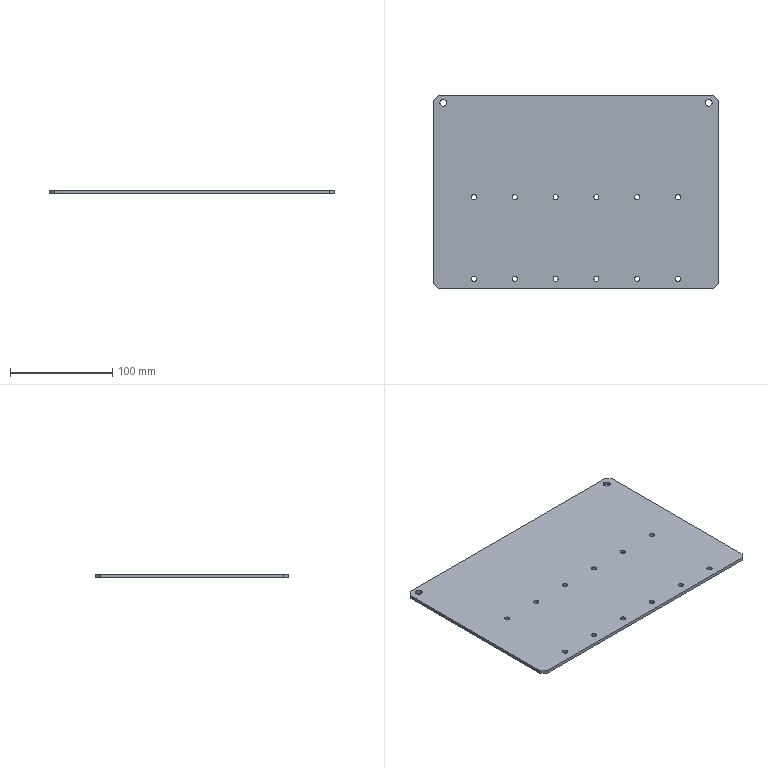Part | STEP file | J014-EBZ05-12-06-Part-1 | 1 solid | 38 faces | box 280 x 190 x 3.2 mm | volume 169094 mm3 | cylinder 28 | plane 10 | commonest cylinder face diameters 5 x24 6.8 x4
STEP:
#1=CARTESIAN_POINT('',(240.,12.5,3.2));
#2=VERTEX_POINT('',#1);
#3=CARTESIAN_POINT('',(240.,7.5,3.2));
#4=VERTEX_POINT('',#3);
#5=CARTESIAN_POINT('',(240.,10.,3.2));
#6=DIRECTION('',(0.,0.,-1.));
#7=DIRECTION('',(0.,-1.,0.));
#8=AXIS2_PLACEMENT_3D('',#5,#6,#7);
#9=CIRCLE('',#8,2.5);
#10=EDGE_CURVE('',#2,#4,#9,.T.);
#11=ORIENTED_EDGE('',*,*,#10,.F.);
#12=CARTESIAN_POINT('',(240.,12.5,0.));
#13=VERTEX_POINT('',#12);
#14=CARTESIAN_POINT('',(240.,12.5,3.2));
#15=DIRECTION('',(0.,0.,-1.));
#16=VECTOR('',#15,1000.);
#17=LINE('',#14,#16);
#18=EDGE_CURVE('',#2,#13,#17,.T.);
#19=ORIENTED_EDGE('',*,*,#18,.T.);
#20=CARTESIAN_POINT('',(240.,7.5,0.));
#21=VERTEX_POINT('',#20);
#22=CARTESIAN_POINT('',(240.,10.,0.));
#23=DIRECTION('',(0.,0.,1.));
#24=DIRECTION('',(0.,1.,0.));
#25=AXIS2_PLACEMENT_3D('',#22,#23,#24);
#26=CIRCLE('',#25,2.5);
#27=EDGE_CURVE('',#21,#13,#26,.T.);
#28=ORIENTED_EDGE('',*,*,#27,.F.);
#29=CARTESIAN_POINT('',(240.,7.5,3.2));
#30=DIRECTION('',(0.,0.,-1.));
#31=VECTOR('',#30,1000.);
#32=LINE('',#29,#31);
#33=EDGE_CURVE('',#4,#21,#32,.T.);
#34=ORIENTED_EDGE('',*,*,#33,.F.);
#35=EDGE_LOOP('',(#11,#19,#28,#34));
#36=FACE_OUTER_BOUND('',#35,.T.);
#37=CARTESIAN_POINT('',(240.,10.,3.2));
#38=DIRECTION('',(0.,0.,-1.));
#39=DIRECTION('',(0.,-1.,0.));
#40=AXIS2_PLACEMENT_3D('',#37,#38,#39);
#41=CYLINDRICAL_SURFACE('',#40,2.5);
#42=ADVANCED_FACE('',(#36),#41,.F.);
#43=CARTESIAN_POINT('',(240.,92.5,3.2));
#44=VERTEX_POINT('',#43);
#45=CARTESIAN_POINT('',(240.,87.5,3.2));
#46=VERTEX_POINT('',#45);
#47=CARTESIAN_POINT('',(240.,90.,3.2));
#48=DIRECTION('',(0.,0.,-1.));
#49=DIRECTION('',(0.,-1.,0.));
#50=AXIS2_PLACEMENT_3D('',#47,#48,#49);
#51=CIRCLE('',#50,2.5);
#52=EDGE_CURVE('',#44,#46,#51,.T.);
#53=ORIENTED_EDGE('',*,*,#52,.F.);
#54=CARTESIAN_POINT('',(240.,92.5,0.));
#55=VERTEX_POINT('',#54);
#56=CARTESIAN_POINT('',(240.,92.5,3.2));
#57=DIRECTION('',(0.,0.,-1.));
#58=VECTOR('',#57,1000.);
#59=LINE('',#56,#58);
#60=EDGE_CURVE('',#44,#55,#59,.T.);
#61=ORIENTED_EDGE('',*,*,#60,.T.);
#62=CARTESIAN_POINT('',(240.,87.5,0.));
#63=VERTEX_POINT('',#62);
#64=CARTESIAN_POINT('',(240.,90.,0.));
#65=DIRECTION('',(0.,0.,1.));
#66=DIRECTION('',(0.,1.,0.));
#67=AXIS2_PLACEMENT_3D('',#64,#65,#66);
#68=CIRCLE('',#67,2.5);
#69=EDGE_CURVE('',#63,#55,#68,.T.);
#70=ORIENTED_EDGE('',*,*,#69,.F.);
#71=CARTESIAN_POINT('',(240.,87.5,3.2));
#72=DIRECTION('',(0.,0.,-1.));
#73=VECTOR('',#72,1000.);
#74=LINE('',#71,#73);
#75=EDGE_CURVE('',#46,#63,#74,.T.);
#76=ORIENTED_EDGE('',*,*,#75,.F.);
#77=EDGE_LOOP('',(#53,#61,#70,#76));
#78=FACE_OUTER_BOUND('',#77,.T.);
#79=CARTESIAN_POINT('',(240.,90.,3.2));
#80=DIRECTION('',(0.,0.,-1.));
#81=DIRECTION('',(0.,-1.,0.));
#82=AXIS2_PLACEMENT_3D('',#79,#80,#81);
#83=CYLINDRICAL_SURFACE('',#82,2.5);
#84=ADVANCED_FACE('',(#78),#83,.F.);
#85=CARTESIAN_POINT('',(200.,12.5,3.2));
#86=VERTEX_POINT('',#85);
#87=CARTESIAN_POINT('',(200.,7.5,3.2));
#88=VERTEX_POINT('',#87);
#89=CARTESIAN_POINT('',(200.,10.,3.2));
#90=DIRECTION('',(0.,0.,-1.));
#91=DIRECTION('',(0.,-1.,0.));
#92=AXIS2_PLACEMENT_3D('',#89,#90,#91);
#93=CIRCLE('',#92,2.5);
#94=EDGE_CURVE('',#86,#88,#93,.T.);
#95=ORIENTED_EDGE('',*,*,#94,.F.);
#96=CARTESIAN_POINT('',(200.,12.5,0.));
#97=VERTEX_POINT('',#96);
#98=CARTESIAN_POINT('',(200.,12.5,3.2));
#99=DIRECTION('',(0.,0.,-1.));
#100=VECTOR('',#99,1000.);
#101=LINE('',#98,#100);
#102=EDGE_CURVE('',#86,#97,#101,.T.);
#103=ORIENTED_EDGE('',*,*,#102,.T.);
#104=CARTESIAN_POINT('',(200.,7.5,0.));
#105=VERTEX_POINT('',#104);
#106=CARTESIAN_POINT('',(200.,10.,0.));
#107=DIRECTION('',(0.,0.,1.));
#108=DIRECTION('',(0.,1.,0.));
#109=AXIS2_PLACEMENT_3D('',#106,#107,#108);
#110=CIRCLE('',#109,2.5);
#111=EDGE_CURVE('',#105,#97,#110,.T.);
#112=ORIENTED_EDGE('',*,*,#111,.F.);
#113=CARTESIAN_POINT('',(200.,7.5,3.2));
#114=DIRECTION('',(0.,0.,-1.));
#115=VECTOR('',#114,1000.);
#116=LINE('',#113,#115);
#117=EDGE_CURVE('',#88,#105,#116,.T.);
#118=ORIENTED_EDGE('',*,*,#117,.F.);
#119=EDGE_LOOP('',(#95,#103,#112,#118));
#120=FACE_OUTER_BOUND('',#119,.T.);
#121=CARTESIAN_POINT('',(200.,10.,3.2));
#122=DIRECTION('',(0.,0.,-1.));
#123=DIRECTION('',(0.,-1.,0.));
#124=AXIS2_PLACEMENT_3D('',#121,#122,#123);
#125=CYLINDRICAL_SURFACE('',#124,2.5);
#126=ADVANCED_FACE('',(#120),#125,.F.);
#127=CARTESIAN_POINT('',(200.,92.5,3.2));
#128=VERTEX_POINT('',#127);
#129=CARTESIAN_POINT('',(200.,87.5,3.2));
#130=VERTEX_POINT('',#129);
#131=CARTESIAN_POINT('',(200.,90.,3.2));
#132=DIRECTION('',(0.,0.,-1.));
#133=DIRECTION('',(0.,-1.,0.));
#134=AXIS2_PLACEMENT_3D('',#131,#132,#133);
#135=CIRCLE('',#134,2.5);
#136=EDGE_CURVE('',#128,#130,#135,.T.);
#137=ORIENTED_EDGE('',*,*,#136,.F.);
#138=CARTESIAN_POINT('',(200.,92.5,0.));
#139=VERTEX_POINT('',#138);
#140=CARTESIAN_POINT('',(200.,92.5,3.2));
#141=DIRECTION('',(0.,0.,-1.));
#142=VECTOR('',#141,1000.);
#143=LINE('',#140,#142);
#144=EDGE_CURVE('',#128,#139,#143,.T.);
#145=ORIENTED_EDGE('',*,*,#144,.T.);
#146=CARTESIAN_POINT('',(200.,87.5,0.));
#147=VERTEX_POINT('',#146);
#148=CARTESIAN_POINT('',(200.,90.,0.));
#149=DIRECTION('',(0.,0.,1.));
#150=DIRECTION('',(0.,1.,0.));
#151=AXIS2_PLACEMENT_3D('',#148,#149,#150);
#152=CIRCLE('',#151,2.5);
#153=EDGE_CURVE('',#147,#139,#152,.T.);
#154=ORIENTED_EDGE('',*,*,#153,.F.);
#155=CARTESIAN_POINT('',(200.,87.5,3.2));
#156=DIRECTION('',(0.,0.,-1.));
#157=VECTOR('',#156,1000.);
#158=LINE('',#155,#157);
#159=EDGE_CURVE('',#130,#147,#158,.T.);
#160=ORIENTED_EDGE('',*,*,#159,.F.);
#161=EDGE_LOOP('',(#137,#145,#154,#160));
#162=FACE_OUTER_BOUND('',#161,.T.);
#163=CARTESIAN_POINT('',(200.,90.,3.2));
#164=DIRECTION('',(0.,0.,-1.));
#165=DIRECTION('',(0.,-1.,0.));
#166=AXIS2_PLACEMENT_3D('',#163,#164,#165);
#167=CYLINDRICAL_SURFACE('',#166,2.5);
#168=ADVANCED_FACE('',(#162),#167,.F.);
#169=CARTESIAN_POINT('',(160.,12.5,3.2));
#170=VERTEX_POINT('',#169);
#171=CARTESIAN_POINT('',(160.,7.5,3.2));
#172=VERTEX_POINT('',#171);
#173=CARTESIAN_POINT('',(160.,10.,3.2));
#174=DIRECTION('',(0.,0.,-1.));
#175=DIRECTION('',(0.,-1.,0.));
#176=AXIS2_PLACEMENT_3D('',#173,#174,#175);
#177=CIRCLE('',#176,2.5);
#178=EDGE_CURVE('',#170,#172,#177,.T.);
#179=ORIENTED_EDGE('',*,*,#178,.F.);
#180=CARTESIAN_POINT('',(160.,12.5,0.));
#181=VERTEX_POINT('',#180);
#182=CARTESIAN_POINT('',(160.,12.5,3.2));
#183=DIRECTION('',(0.,0.,-1.));
#184=VECTOR('',#183,1000.);
#185=LINE('',#182,#184);
#186=EDGE_CURVE('',#170,#181,#185,.T.);
#187=ORIENTED_EDGE('',*,*,#186,.T.);
#188=CARTESIAN_POINT('',(160.,7.5,0.));
#189=VERTEX_POINT('',#188);
#190=CARTESIAN_POINT('',(160.,10.,0.));
#191=DIRECTION('',(0.,0.,1.));
#192=DIRECTION('',(0.,1.,0.));
#193=AXIS2_PLACEMENT_3D('',#190,#191,#192);
#194=CIRCLE('',#193,2.5);
#195=EDGE_CURVE('',#189,#181,#194,.T.);
#196=ORIENTED_EDGE('',*,*,#195,.F.);
#197=CARTESIAN_POINT('',(160.,7.5,3.2));
#198=DIRECTION('',(0.,0.,-1.));
#199=VECTOR('',#198,1000.);
#200=LINE('',#197,#199);
#201=EDGE_CURVE('',#172,#189,#200,.T.);
#202=ORIENTED_EDGE('',*,*,#201,.F.);
#203=EDGE_LOOP('',(#179,#187,#196,#202));
#204=FACE_OUTER_BOUND('',#203,.T.);
#205=CARTESIAN_POINT('',(160.,10.,3.2));
#206=DIRECTION('',(0.,0.,-1.));
#207=DIRECTION('',(0.,-1.,0.));
#208=AXIS2_PLACEMENT_3D('',#205,#206,#207);
#209=CYLINDRICAL_SURFACE('',#208,2.5);
#210=ADVANCED_FACE('',(#204),#209,.F.);
#211=CARTESIAN_POINT('',(160.,92.5,3.2));
#212=VERTEX_POINT('',#211);
#213=CARTESIAN_POINT('',(160.,87.5,3.2));
#214=VERTEX_POINT('',#213);
#215=CARTESIAN_POINT('',(160.,90.,3.2));
#216=DIRECTION('',(0.,0.,-1.));
#217=DIRECTION('',(0.,-1.,0.));
#218=AXIS2_PLACEMENT_3D('',#215,#216,#217);
#219=CIRCLE('',#218,2.5);
#220=EDGE_CURVE('',#212,#214,#219,.T.);
#221=ORIENTED_EDGE('',*,*,#220,.F.);
#222=CARTESIAN_POINT('',(160.,92.5,0.));
#223=VERTEX_POINT('',#222);
#224=CARTESIAN_POINT('',(160.,92.5,3.2));
#225=DIRECTION('',(0.,0.,-1.));
#226=VECTOR('',#225,1000.);
#227=LINE('',#224,#226);
#228=EDGE_CURVE('',#212,#223,#227,.T.);
#229=ORIENTED_EDGE('',*,*,#228,.T.);
#230=CARTESIAN_POINT('',(160.,87.5,0.));
#231=VERTEX_POINT('',#230);
#232=CARTESIAN_POINT('',(160.,90.,0.));
#233=DIRECTION('',(0.,0.,1.));
#234=DIRECTION('',(0.,1.,0.));
#235=AXIS2_PLACEMENT_3D('',#232,#233,#234);
#236=CIRCLE('',#235,2.5);
#237=EDGE_CURVE('',#231,#223,#236,.T.);
#238=ORIENTED_EDGE('',*,*,#237,.F.);
#239=CARTESIAN_POINT('',(160.,87.5,3.2));
#240=DIRECTION('',(0.,0.,-1.));
#241=VECTOR('',#240,1000.);
#242=LINE('',#239,#241);
#243=EDGE_CURVE('',#214,#231,#242,.T.);
#244=ORIENTED_EDGE('',*,*,#243,.F.);
#245=EDGE_LOOP('',(#221,#229,#238,#244));
#246=FACE_OUTER_BOUND('',#245,.T.);
#247=CARTESIAN_POINT('',(160.,90.,3.2));
#248=DIRECTION('',(0.,0.,-1.));
#249=DIRECTION('',(0.,-1.,0.));
#250=AXIS2_PLACEMENT_3D('',#247,#248,#249);
#251=CYLINDRICAL_SURFACE('',#250,2.5);
#252=ADVANCED_FACE('',(#246),#251,.F.);
#253=CARTESIAN_POINT('',(120.,12.5,3.2));
#254=VERTEX_POINT('',#253);
#255=CARTESIAN_POINT('',(120.,7.5,3.2));
#256=VERTEX_POINT('',#255);
#257=CARTESIAN_POINT('',(120.,10.,3.2));
#258=DIRECTION('',(0.,0.,-1.));
#259=DIRECTION('',(0.,-1.,0.));
#260=AXIS2_PLACEMENT_3D('',#257,#258,#259);
#261=CIRCLE('',#260,2.5);
#262=EDGE_CURVE('',#254,#256,#261,.T.);
#263=ORIENTED_EDGE('',*,*,#262,.F.);
#264=CARTESIAN_POINT('',(120.,12.5,0.));
#265=VERTEX_POINT('',#264);
#266=CARTESIAN_POINT('',(120.,12.5,3.2));
#267=DIRECTION('',(0.,0.,-1.));
#268=VECTOR('',#267,1000.);
#269=LINE('',#266,#268);
#270=EDGE_CURVE('',#254,#265,#269,.T.);
#271=ORIENTED_EDGE('',*,*,#270,.T.);
#272=CARTESIAN_POINT('',(120.,7.5,0.));
#273=VERTEX_POINT('',#272);
#274=CARTESIAN_POINT('',(120.,10.,0.));
#275=DIRECTION('',(0.,0.,1.));
#276=DIRECTION('',(0.,1.,0.));
#277=AXIS2_PLACEMENT_3D('',#274,#275,#276);
#278=CIRCLE('',#277,2.5);
#279=EDGE_CURVE('',#273,#265,#278,.T.);
#280=ORIENTED_EDGE('',*,*,#279,.F.);
#281=CARTESIAN_POINT('',(120.,7.5,3.2));
#282=DIRECTION('',(0.,0.,-1.));
#283=VECTOR('',#282,1000.);
#284=LINE('',#281,#283);
#285=EDGE_CURVE('',#256,#273,#284,.T.);
#286=ORIENTED_EDGE('',*,*,#285,.F.);
#287=EDGE_LOOP('',(#263,#271,#280,#286));
#288=FACE_OUTER_BOUND('',#287,.T.);
#289=CARTESIAN_POINT('',(120.,10.,3.2));
#290=DIRECTION('',(0.,0.,-1.));
#291=DIRECTION('',(0.,-1.,0.));
#292=AXIS2_PLACEMENT_3D('',#289,#290,#291);
#293=CYLINDRICAL_SURFACE('',#292,2.5);
#294=ADVANCED_FACE('',(#288),#293,.F.);
#295=CARTESIAN_POINT('',(120.,92.5,3.2));
#296=VERTEX_POINT('',#295);
#297=CARTESIAN_POINT('',(120.,87.5,3.2));
#298=VERTEX_POINT('',#297);
#299=CARTESIAN_POINT('',(120.,90.,3.2));
#300=DIRECTION('',(0.,0.,-1.));
#301=DIRECTION('',(0.,-1.,0.));
#302=AXIS2_PLACEMENT_3D('',#299,#300,#301);
#303=CIRCLE('',#302,2.5);
#304=EDGE_CURVE('',#296,#298,#303,.T.);
#305=ORIENTED_EDGE('',*,*,#304,.F.);
#306=CARTESIAN_POINT('',(120.,92.5,0.));
#307=VERTEX_POINT('',#306);
#308=CARTESIAN_POINT('',(120.,92.5,3.2));
#309=DIRECTION('',(0.,0.,-1.));
#310=VECTOR('',#309,1000.);
#311=LINE('',#308,#310);
#312=EDGE_CURVE('',#296,#307,#311,.T.);
#313=ORIENTED_EDGE('',*,*,#312,.T.);
#314=CARTESIAN_POINT('',(120.,87.5,0.));
#315=VERTEX_POINT('',#314);
#316=CARTESIAN_POINT('',(120.,90.,0.));
#317=DIRECTION('',(0.,0.,1.));
#318=DIRECTION('',(0.,1.,0.));
#319=AXIS2_PLACEMENT_3D('',#316,#317,#318);
#320=CIRCLE('',#319,2.5);
#321=EDGE_CURVE('',#315,#307,#320,.T.);
#322=ORIENTED_EDGE('',*,*,#321,.F.);
#323=CARTESIAN_POINT('',(120.,87.5,3.2));
#324=DIRECTION('',(0.,0.,-1.));
#325=VECTOR('',#324,1000.);
#326=LINE('',#323,#325);
#327=EDGE_CURVE('',#298,#315,#326,.T.);
#328=ORIENTED_EDGE('',*,*,#327,.F.);
#329=EDGE_LOOP('',(#305,#313,#322,#328));
#330=FACE_OUTER_BOUND('',#329,.T.);
#331=CARTESIAN_POINT('',(120.,90.,3.2));
#332=DIRECTION('',(0.,0.,-1.));
#333=DIRECTION('',(0.,-1.,0.));
#334=AXIS2_PLACEMENT_3D('',#331,#332,#333);
#335=CYLINDRICAL_SURFACE('',#334,2.5);
#336=ADVANCED_FACE('',(#330),#335,.F.);
#337=CARTESIAN_POINT('',(80.,12.5,3.2));
#338=VERTEX_POINT('',#337);
#339=CARTESIAN_POINT('',(80.,7.5,3.2));
#340=VERTEX_POINT('',#339);
#341=CARTESIAN_POINT('',(80.,10.,3.2));
#342=DIRECTION('',(0.,0.,-1.));
#343=DIRECTION('',(0.,-1.,0.));
#344=AXIS2_PLACEMENT_3D('',#341,#342,#343);
#345=CIRCLE('',#344,2.5);
#346=EDGE_CURVE('',#338,#340,#345,.T.);
#347=ORIENTED_EDGE('',*,*,#346,.F.);
#348=CARTESIAN_POINT('',(80.,12.5,0.));
#349=VERTEX_POINT('',#348);
#350=CARTESIAN_POINT('',(80.,12.5,3.2));
#351=DIRECTION('',(0.,0.,-1.));
#352=VECTOR('',#351,1000.);
#353=LINE('',#350,#352);
#354=EDGE_CURVE('',#338,#349,#353,.T.);
#355=ORIENTED_EDGE('',*,*,#354,.T.);
#356=CARTESIAN_POINT('',(80.,7.5,0.));
#357=VERTEX_POINT('',#356);
#358=CARTESIAN_POINT('',(80.,10.,0.));
#359=DIRECTION('',(0.,0.,1.));
#360=DIRECTION('',(0.,1.,0.));
#361=AXIS2_PLACEMENT_3D('',#358,#359,#360);
#362=CIRCLE('',#361,2.5);
#363=EDGE_CURVE('',#357,#349,#362,.T.);
#364=ORIENTED_EDGE('',*,*,#363,.F.);
#365=CARTESIAN_POINT('',(80.,7.5,3.2));
#366=DIRECTION('',(0.,0.,-1.));
#367=VECTOR('',#366,1000.);
#368=LINE('',#365,#367);
#369=EDGE_CURVE('',#340,#357,#368,.T.);
#370=ORIENTED_EDGE('',*,*,#369,.F.);
#371=EDGE_LOOP('',(#347,#355,#364,#370));
#372=FACE_OUTER_BOUND('',#371,.T.);
#373=CARTESIAN_POINT('',(80.,10.,3.2));
#374=DIRECTION('',(0.,0.,-1.));
#375=DIRECTION('',(0.,-1.,0.));
#376=AXIS2_PLACEMENT_3D('',#373,#374,#375);
#377=CYLINDRICAL_SURFACE('',#376,2.5);
#378=ADVANCED_FACE('',(#372),#377,.F.);
#379=CARTESIAN_POINT('',(80.,92.5,3.2));
#380=VERTEX_POINT('',#379);
#381=CARTESIAN_POINT('',(80.,87.5,3.2));
#382=VERTEX_POINT('',#381);
#383=CARTESIAN_POINT('',(80.,90.,3.2));
#384=DIRECTION('',(0.,0.,-1.));
#385=DIRECTION('',(0.,-1.,0.));
#386=AXIS2_PLACEMENT_3D('',#383,#384,#385);
#387=CIRCLE('',#386,2.5);
#388=EDGE_CURVE('',#380,#382,#387,.T.);
#389=ORIENTED_EDGE('',*,*,#388,.F.);
#390=CARTESIAN_POINT('',(80.,92.5,0.));
#391=VERTEX_POINT('',#390);
#392=CARTESIAN_POINT('',(80.,92.5,3.2));
#393=DIRECTION('',(0.,0.,-1.));
#394=VECTOR('',#393,1000.);
#395=LINE('',#392,#394);
#396=EDGE_CURVE('',#380,#391,#395,.T.);
#397=ORIENTED_EDGE('',*,*,#396,.T.);
#398=CARTESIAN_POINT('',(80.,87.5,0.));
#399=VERTEX_POINT('',#398);
#400=CARTESIAN_POINT('',(80.,90.,0.));
#401=DIRECTION('',(0.,0.,1.));
#402=DIRECTION('',(0.,1.,0.));
#403=AXIS2_PLACEMENT_3D('',#400,#401,#402);
#404=CIRCLE('',#403,2.5);
#405=EDGE_CURVE('',#399,#391,#404,.T.);
#406=ORIENTED_EDGE('',*,*,#405,.F.);
#407=CARTESIAN_POINT('',(80.,87.5,3.2));
#408=DIRECTION('',(0.,0.,-1.));
#409=VECTOR('',#408,1000.);
#410=LINE('',#407,#409);
#411=EDGE_CURVE('',#382,#399,#410,.T.);
#412=ORIENTED_EDGE('',*,*,#411,.F.);
#413=EDGE_LOOP('',(#389,#397,#406,#412));
#414=FACE_OUTER_BOUND('',#413,.T.);
#415=CARTESIAN_POINT('',(80.,90.,3.2));
#416=DIRECTION('',(0.,0.,-1.));
#417=DIRECTION('',(0.,-1.,0.));
#418=AXIS2_PLACEMENT_3D('',#415,#416,#417);
#419=CYLINDRICAL_SURFACE('',#418,2.5);
#420=ADVANCED_FACE('',(#414),#419,.F.);
#421=CARTESIAN_POINT('',(40.,12.5,3.2));
#422=VERTEX_POINT('',#421);
#423=CARTESIAN_POINT('',(40.,7.5,3.2));
#424=VERTEX_POINT('',#423);
#425=CARTESIAN_POINT('',(40.,10.,3.2));
#426=DIRECTION('',(0.,0.,-1.));
#427=DIRECTION('',(0.,-1.,0.));
#428=AXIS2_PLACEMENT_3D('',#425,#426,#427);
#429=CIRCLE('',#428,2.5);
#430=EDGE_CURVE('',#422,#424,#429,.T.);
#431=ORIENTED_EDGE('',*,*,#430,.F.);
#432=CARTESIAN_POINT('',(40.,12.5,0.));
#433=VERTEX_POINT('',#432);
#434=CARTESIAN_POINT('',(40.,12.5,3.2));
#435=DIRECTION('',(0.,0.,-1.));
#436=VECTOR('',#435,1000.);
#437=LINE('',#434,#436);
#438=EDGE_CURVE('',#422,#433,#437,.T.);
#439=ORIENTED_EDGE('',*,*,#438,.T.);
#440=CARTESIAN_POINT('',(40.,7.5,0.));
#441=VERTEX_POINT('',#440);
#442=CARTESIAN_POINT('',(40.,10.,0.));
#443=DIRECTION('',(0.,0.,1.));
#444=DIRECTION('',(0.,1.,0.));
#445=AXIS2_PLACEMENT_3D('',#442,#443,#444);
#446=CIRCLE('',#445,2.5);
#447=EDGE_CURVE('',#441,#433,#446,.T.);
#448=ORIENTED_EDGE('',*,*,#447,.F.);
#449=CARTESIAN_POINT('',(40.,7.5,3.2));
#450=DIRECTION('',(0.,0.,-1.));
#451=VECTOR('',#450,1000.);
#452=LINE('',#449,#451);
#453=EDGE_CURVE('',#424,#441,#452,.T.);
#454=ORIENTED_EDGE('',*,*,#453,.F.);
#455=EDGE_LOOP('',(#431,#439,#448,#454));
#456=FACE_OUTER_BOUND('',#455,.T.);
#457=CARTESIAN_POINT('',(40.,10.,3.2));
#458=DIRECTION('',(0.,0.,-1.));
#459=DIRECTION('',(0.,-1.,0.));
#460=AXIS2_PLACEMENT_3D('',#457,#458,#459);
#461=CYLINDRICAL_SURFACE('',#460,2.5);
#462=ADVANCED_FACE('',(#456),#461,.F.);
#463=CARTESIAN_POINT('',(40.,92.5,3.2));
#464=VERTEX_POINT('',#463);
#465=CARTESIAN_POINT('',(40.,87.5,3.2));
#466=VERTEX_POINT('',#465);
#467=CARTESIAN_POINT('',(40.,90.,3.2));
#468=DIRECTION('',(0.,0.,-1.));
#469=DIRECTION('',(0.,-1.,0.));
#470=AXIS2_PLACEMENT_3D('',#467,#468,#469);
#471=CIRCLE('',#470,2.5);
#472=EDGE_CURVE('',#464,#466,#471,.T.);
#473=ORIENTED_EDGE('',*,*,#472,.F.);
#474=CARTESIAN_POINT('',(40.,92.5,0.));
#475=VERTEX_POINT('',#474);
#476=CARTESIAN_POINT('',(40.,92.5,3.2));
#477=DIRECTION('',(0.,0.,-1.));
#478=VECTOR('',#477,1000.);
#479=LINE('',#476,#478);
#480=EDGE_CURVE('',#464,#475,#479,.T.);
#481=ORIENTED_EDGE('',*,*,#480,.T.);
#482=CARTESIAN_POINT('',(40.,87.5,0.));
#483=VERTEX_POINT('',#482);
#484=CARTESIAN_POINT('',(40.,90.,0.));
#485=DIRECTION('',(0.,0.,1.));
#486=DIRECTION('',(0.,1.,0.));
#487=AXIS2_PLACEMENT_3D('',#484,#485,#486);
#488=CIRCLE('',#487,2.5);
#489=EDGE_CURVE('',#483,#475,#488,.T.);
#490=ORIENTED_EDGE('',*,*,#489,.F.);
#491=CARTESIAN_POINT('',(40.,87.5,3.2));
#492=DIRECTION('',(0.,0.,-1.));
#493=VECTOR('',#492,1000.);
#494=LINE('',#491,#493);
#495=EDGE_CURVE('',#466,#483,#494,.T.);
#496=ORIENTED_EDGE('',*,*,#495,.F.);
#497=EDGE_LOOP('',(#473,#481,#490,#496));
#498=FACE_OUTER_BOUND('',#497,.T.);
#499=CARTESIAN_POINT('',(40.,90.,3.2));
#500=DIRECTION('',(0.,0.,-1.));
#501=DIRECTION('',(0.,-1.,0.));
#502=AXIS2_PLACEMENT_3D('',#499,#500,#501);
#503=CYLINDRICAL_SURFACE('',#502,2.5);
#504=ADVANCED_FACE('',(#498),#503,.F.);
#505=CARTESIAN_POINT('',(270.,185.9,3.2));
#506=VERTEX_POINT('',#505);
#507=CARTESIAN_POINT('',(270.,179.1,3.2));
#508=VERTEX_POINT('',#507);
#509=CARTESIAN_POINT('',(270.,182.5,3.2));
#510=DIRECTION('',(0.,0.,-1.));
#511=DIRECTION('',(0.,-1.,0.));
#512=AXIS2_PLACEMENT_3D('',#509,#510,#511);
#513=CIRCLE('',#512,3.4);
#514=EDGE_CURVE('',#506,#508,#513,.T.);
#515=ORIENTED_EDGE('',*,*,#514,.F.);
#516=CARTESIAN_POINT('',(270.,185.9,0.));
#517=VERTEX_POINT('',#516);
#518=CARTESIAN_POINT('',(270.,185.9,3.2));
#519=DIRECTION('',(0.,0.,-1.));
#520=VECTOR('',#519,1000.);
#521=LINE('',#518,#520);
#522=EDGE_CURVE('',#506,#517,#521,.T.);
#523=ORIENTED_EDGE('',*,*,#522,.T.);
#524=CARTESIAN_POINT('',(270.,179.1,0.));
#525=VERTEX_POINT('',#524);
#526=CARTESIAN_POINT('',(270.,182.5,0.));
#527=DIRECTION('',(0.,0.,1.));
#528=DIRECTION('',(0.,1.,0.));
#529=AXIS2_PLACEMENT_3D('',#526,#527,#528);
#530=CIRCLE('',#529,3.4);
#531=EDGE_CURVE('',#525,#517,#530,.T.);
#532=ORIENTED_EDGE('',*,*,#531,.F.);
#533=CARTESIAN_POINT('',(270.,179.1,3.2));
#534=DIRECTION('',(0.,0.,-1.));
#535=VECTOR('',#534,1000.);
#536=LINE('',#533,#535);
#537=EDGE_CURVE('',#508,#525,#536,.T.);
#538=ORIENTED_EDGE('',*,*,#537,.F.);
#539=EDGE_LOOP('',(#515,#523,#532,#538));
#540=FACE_OUTER_BOUND('',#539,.T.);
#541=CARTESIAN_POINT('',(270.,182.5,3.2));
#542=DIRECTION('',(0.,0.,-1.));
#543=DIRECTION('',(0.,-1.,0.));
#544=AXIS2_PLACEMENT_3D('',#541,#542,#543);
#545=CYLINDRICAL_SURFACE('',#544,3.4);
#546=ADVANCED_FACE('',(#540),#545,.F.);
#547=CARTESIAN_POINT('',(10.,185.9,3.2));
#548=VERTEX_POINT('',#547);
#549=CARTESIAN_POINT('',(10.,179.1,3.2));
#550=VERTEX_POINT('',#549);
#551=CARTESIAN_POINT('',(10.,182.5,3.2));
#552=DIRECTION('',(0.,0.,-1.));
#553=DIRECTION('',(0.,-1.,0.));
#554=AXIS2_PLACEMENT_3D('',#551,#552,#553);
#555=CIRCLE('',#554,3.4);
#556=EDGE_CURVE('',#548,#550,#555,.T.);
#557=ORIENTED_EDGE('',*,*,#556,.F.);
#558=CARTESIAN_POINT('',(10.,185.9,0.));
#559=VERTEX_POINT('',#558);
#560=CARTESIAN_POINT('',(10.,185.9,3.2));
#561=DIRECTION('',(0.,0.,-1.));
#562=VECTOR('',#561,1000.);
#563=LINE('',#560,#562);
#564=EDGE_CURVE('',#548,#559,#563,.T.);
#565=ORIENTED_EDGE('',*,*,#564,.T.);
#566=CARTESIAN_POINT('',(10.,179.1,0.));
#567=VERTEX_POINT('',#566);
#568=CARTESIAN_POINT('',(10.,182.5,0.));
#569=DIRECTION('',(0.,0.,1.));
#570=DIRECTION('',(0.,1.,0.));
#571=AXIS2_PLACEMENT_3D('',#568,#569,#570);
#572=CIRCLE('',#571,3.4);
#573=EDGE_CURVE('',#567,#559,#572,.T.);
#574=ORIENTED_EDGE('',*,*,#573,.F.);
#575=CARTESIAN_POINT('',(10.,179.1,3.2));
#576=DIRECTION('',(0.,0.,-1.));
#577=VECTOR('',#576,1000.);
#578=LINE('',#575,#577);
#579=EDGE_CURVE('',#550,#567,#578,.T.);
#580=ORIENTED_EDGE('',*,*,#579,.F.);
#581=EDGE_LOOP('',(#557,#565,#574,#580));
#582=FACE_OUTER_BOUND('',#581,.T.);
#583=CARTESIAN_POINT('',(10.,182.5,3.2));
#584=DIRECTION('',(0.,0.,-1.));
#585=DIRECTION('',(0.,-1.,0.));
#586=AXIS2_PLACEMENT_3D('',#583,#584,#585);
#587=CYLINDRICAL_SURFACE('',#586,3.4);
#588=ADVANCED_FACE('',(#582),#587,.F.);
#589=CARTESIAN_POINT('',(240.,10.,3.2));
#590=DIRECTION('',(0.,0.,-1.));
#591=DIRECTION('',(0.,-1.,0.));
#592=AXIS2_PLACEMENT_3D('',#589,#590,#591);
#593=CIRCLE('',#592,2.5);
#594=EDGE_CURVE('',#4,#2,#593,.T.);
#595=ORIENTED_EDGE('',*,*,#594,.T.);
#596=ORIENTED_EDGE('',*,*,#10,.T.);
#597=EDGE_LOOP('',(#595,#596));
#598=FACE_BOUND('',#597,.T.);
#599=CARTESIAN_POINT('',(240.,90.,3.2));
#600=DIRECTION('',(0.,0.,-1.));
#601=DIRECTION('',(0.,-1.,0.));
#602=AXIS2_PLACEMENT_3D('',#599,#600,#601);
#603=CIRCLE('',#602,2.5);
#604=EDGE_CURVE('',#46,#44,#603,.T.);
#605=ORIENTED_EDGE('',*,*,#604,.T.);
#606=ORIENTED_EDGE('',*,*,#52,.T.);
#607=EDGE_LOOP('',(#605,#606));
#608=FACE_BOUND('',#607,.T.);
#609=CARTESIAN_POINT('',(200.,10.,3.2));
#610=DIRECTION('',(0.,0.,-1.));
#611=DIRECTION('',(0.,-1.,0.));
#612=AXIS2_PLACEMENT_3D('',#609,#610,#611);
#613=CIRCLE('',#612,2.5);
#614=EDGE_CURVE('',#88,#86,#613,.T.);
#615=ORIENTED_EDGE('',*,*,#614,.T.);
#616=ORIENTED_EDGE('',*,*,#94,.T.);
#617=EDGE_LOOP('',(#615,#616));
#618=FACE_BOUND('',#617,.T.);
#619=CARTESIAN_POINT('',(200.,90.,3.2));
#620=DIRECTION('',(0.,0.,-1.));
#621=DIRECTION('',(0.,-1.,0.));
#622=AXIS2_PLACEMENT_3D('',#619,#620,#621);
#623=CIRCLE('',#622,2.5);
#624=EDGE_CURVE('',#130,#128,#623,.T.);
#625=ORIENTED_EDGE('',*,*,#624,.T.);
#626=ORIENTED_EDGE('',*,*,#136,.T.);
#627=EDGE_LOOP('',(#625,#626));
#628=FACE_BOUND('',#627,.T.);
#629=CARTESIAN_POINT('',(160.,10.,3.2));
#630=DIRECTION('',(0.,0.,-1.));
#631=DIRECTION('',(0.,-1.,0.));
#632=AXIS2_PLACEMENT_3D('',#629,#630,#631);
#633=CIRCLE('',#632,2.5);
#634=EDGE_CURVE('',#172,#170,#633,.T.);
#635=ORIENTED_EDGE('',*,*,#634,.T.);
#636=ORIENTED_EDGE('',*,*,#178,.T.);
#637=EDGE_LOOP('',(#635,#636));
#638=FACE_BOUND('',#637,.T.);
#639=CARTESIAN_POINT('',(160.,90.,3.2));
#640=DIRECTION('',(0.,0.,-1.));
#641=DIRECTION('',(0.,-1.,0.));
#642=AXIS2_PLACEMENT_3D('',#639,#640,#641);
#643=CIRCLE('',#642,2.5);
#644=EDGE_CURVE('',#214,#212,#643,.T.);
#645=ORIENTED_EDGE('',*,*,#644,.T.);
#646=ORIENTED_EDGE('',*,*,#220,.T.);
#647=EDGE_LOOP('',(#645,#646));
#648=FACE_BOUND('',#647,.T.);
#649=CARTESIAN_POINT('',(120.,10.,3.2));
#650=DIRECTION('',(0.,0.,-1.));
#651=DIRECTION('',(0.,-1.,0.));
#652=AXIS2_PLACEMENT_3D('',#649,#650,#651);
#653=CIRCLE('',#652,2.5);
#654=EDGE_CURVE('',#256,#254,#653,.T.);
#655=ORIENTED_EDGE('',*,*,#654,.T.);
#656=ORIENTED_EDGE('',*,*,#262,.T.);
#657=EDGE_LOOP('',(#655,#656));
#658=FACE_BOUND('',#657,.T.);
#659=CARTESIAN_POINT('',(120.,90.,3.2));
#660=DIRECTION('',(0.,0.,-1.));
#661=DIRECTION('',(0.,-1.,0.));
#662=AXIS2_PLACEMENT_3D('',#659,#660,#661);
#663=CIRCLE('',#662,2.5);
#664=EDGE_CURVE('',#298,#296,#663,.T.);
#665=ORIENTED_EDGE('',*,*,#664,.T.);
#666=ORIENTED_EDGE('',*,*,#304,.T.);
#667=EDGE_LOOP('',(#665,#666));
#668=FACE_BOUND('',#667,.T.);
#669=CARTESIAN_POINT('',(80.,10.,3.2));
#670=DIRECTION('',(0.,0.,-1.));
#671=DIRECTION('',(0.,-1.,0.));
#672=AXIS2_PLACEMENT_3D('',#669,#670,#671);
#673=CIRCLE('',#672,2.5);
#674=EDGE_CURVE('',#340,#338,#673,.T.);
#675=ORIENTED_EDGE('',*,*,#674,.T.);
#676=ORIENTED_EDGE('',*,*,#346,.T.);
#677=EDGE_LOOP('',(#675,#676));
#678=FACE_BOUND('',#677,.T.);
#679=CARTESIAN_POINT('',(80.,90.,3.2));
#680=DIRECTION('',(0.,0.,-1.));
#681=DIRECTION('',(0.,-1.,0.));
#682=AXIS2_PLACEMENT_3D('',#679,#680,#681);
#683=CIRCLE('',#682,2.5);
#684=EDGE_CURVE('',#382,#380,#683,.T.);
#685=ORIENTED_EDGE('',*,*,#684,.T.);
#686=ORIENTED_EDGE('',*,*,#388,.T.);
#687=EDGE_LOOP('',(#685,#686));
#688=FACE_BOUND('',#687,.T.);
#689=CARTESIAN_POINT('',(40.,10.,3.2));
#690=DIRECTION('',(0.,0.,-1.));
#691=DIRECTION('',(0.,-1.,0.));
#692=AXIS2_PLACEMENT_3D('',#689,#690,#691);
#693=CIRCLE('',#692,2.5);
#694=EDGE_CURVE('',#424,#422,#693,.T.);
#695=ORIENTED_EDGE('',*,*,#694,.T.);
#696=ORIENTED_EDGE('',*,*,#430,.T.);
#697=EDGE_LOOP('',(#695,#696));
#698=FACE_BOUND('',#697,.T.);
#699=CARTESIAN_POINT('',(40.,90.,3.2));
#700=DIRECTION('',(0.,0.,-1.));
#701=DIRECTION('',(0.,-1.,0.));
#702=AXIS2_PLACEMENT_3D('',#699,#700,#701);
#703=CIRCLE('',#702,2.5);
#704=EDGE_CURVE('',#466,#464,#703,.T.);
#705=ORIENTED_EDGE('',*,*,#704,.T.);
#706=ORIENTED_EDGE('',*,*,#472,.T.);
#707=EDGE_LOOP('',(#705,#706));
#708=FACE_BOUND('',#707,.T.);
#709=CARTESIAN_POINT('',(270.,182.5,3.2));
#710=DIRECTION('',(0.,0.,-1.));
#711=DIRECTION('',(0.,-1.,0.));
#712=AXIS2_PLACEMENT_3D('',#709,#710,#711);
#713=CIRCLE('',#712,3.4);
#714=EDGE_CURVE('',#508,#506,#713,.T.);
#715=ORIENTED_EDGE('',*,*,#714,.T.);
#716=ORIENTED_EDGE('',*,*,#514,.T.);
#717=EDGE_LOOP('',(#715,#716));
#718=FACE_BOUND('',#717,.T.);
#719=CARTESIAN_POINT('',(10.,182.5,3.2));
#720=DIRECTION('',(0.,0.,-1.));
#721=DIRECTION('',(0.,-1.,0.));
#722=AXIS2_PLACEMENT_3D('',#719,#720,#721);
#723=CIRCLE('',#722,3.4);
#724=EDGE_CURVE('',#550,#548,#723,.T.);
#725=ORIENTED_EDGE('',*,*,#724,.T.);
#726=ORIENTED_EDGE('',*,*,#556,.T.);
#727=EDGE_LOOP('',(#725,#726));
#728=FACE_BOUND('',#727,.T.);
#729=CARTESIAN_POINT('',(280.,185.,3.2));
#730=VERTEX_POINT('',#729);
#731=CARTESIAN_POINT('',(280.,5.,3.2));
#732=VERTEX_POINT('',#731);
#733=CARTESIAN_POINT('',(280.,95.,3.2));
#734=DIRECTION('',(0.,-1.,0.));
#735=VECTOR('',#734,1000.);
#736=LINE('',#733,#735);
#737=EDGE_CURVE('',#730,#732,#736,.T.);
#738=ORIENTED_EDGE('',*,*,#737,.F.);
#739=CARTESIAN_POINT('',(275.,190.,3.2));
#740=VERTEX_POINT('',#739);
#741=CARTESIAN_POINT('',(255.,210.,3.2));
#742=DIRECTION('',(-0.7071,0.7071,0.));
#743=VECTOR('',#742,1000.);
#744=LINE('',#741,#743);
#745=EDGE_CURVE('',#730,#740,#744,.T.);
#746=ORIENTED_EDGE('',*,*,#745,.T.);
#747=CARTESIAN_POINT('',(5.,190.,3.2));
#748=VERTEX_POINT('',#747);
#749=CARTESIAN_POINT('',(140.,190.,3.2));
#750=DIRECTION('',(1.,0.,0.));
#751=VECTOR('',#750,1000.);
#752=LINE('',#749,#751);
#753=EDGE_CURVE('',#748,#740,#752,.T.);
#754=ORIENTED_EDGE('',*,*,#753,.F.);
#755=CARTESIAN_POINT('',(0.,185.,3.2));
#756=VERTEX_POINT('',#755);
#757=CARTESIAN_POINT('',(25.,210.,3.2));
#758=DIRECTION('',(-0.7071,-0.7071,0.));
#759=VECTOR('',#758,1000.);
#760=LINE('',#757,#759);
#761=EDGE_CURVE('',#748,#756,#760,.T.);
#762=ORIENTED_EDGE('',*,*,#761,.T.);
#763=CARTESIAN_POINT('',(0.,5.,3.2));
#764=VERTEX_POINT('',#763);
#765=CARTESIAN_POINT('',(0.,95.,3.2));
#766=DIRECTION('',(0.,1.,0.));
#767=VECTOR('',#766,1000.);
#768=LINE('',#765,#767);
#769=EDGE_CURVE('',#764,#756,#768,.T.);
#770=ORIENTED_EDGE('',*,*,#769,.F.);
#771=CARTESIAN_POINT('',(5.,0.,3.2));
#772=VERTEX_POINT('',#771);
#773=CARTESIAN_POINT('',(25.,-20.,3.2));
#774=DIRECTION('',(0.7071,-0.7071,0.));
#775=VECTOR('',#774,1000.);
#776=LINE('',#773,#775);
#777=EDGE_CURVE('',#764,#772,#776,.T.);
#778=ORIENTED_EDGE('',*,*,#777,.T.);
#779=CARTESIAN_POINT('',(275.,0.,3.2));
#780=VERTEX_POINT('',#779);
#781=CARTESIAN_POINT('',(140.,0.,3.2));
#782=DIRECTION('',(-1.,0.,0.));
#783=VECTOR('',#782,1000.);
#784=LINE('',#781,#783);
#785=EDGE_CURVE('',#780,#772,#784,.T.);
#786=ORIENTED_EDGE('',*,*,#785,.F.);
#787=CARTESIAN_POINT('',(255.,-20.,3.2));
#788=DIRECTION('',(0.7071,0.7071,0.));
#789=VECTOR('',#788,1000.);
#790=LINE('',#787,#789);
#791=EDGE_CURVE('',#780,#732,#790,.T.);
#792=ORIENTED_EDGE('',*,*,#791,.T.);
#793=EDGE_LOOP('',(#738,#746,#754,#762,#770,#778,#786,#792));
#794=FACE_OUTER_BOUND('',#793,.T.);
#795=CARTESIAN_POINT('',(140.,95.,3.2));
#796=DIRECTION('',(0.,0.,1.));
#797=DIRECTION('',(-1.,0.,0.));
#798=AXIS2_PLACEMENT_3D('',#795,#796,#797);
#799=PLANE('',#798);
#800=ADVANCED_FACE('',(#598,#608,#618,#628,#638,#648,#658,#668,#678,#688,#698,#708,#718,#728,#794),#799,.T.);
#801=ORIENTED_EDGE('',*,*,#753,.T.);
#802=CARTESIAN_POINT('',(275.,190.,0.));
#803=VERTEX_POINT('',#802);
#804=CARTESIAN_POINT('',(275.,190.,0.));
#805=DIRECTION('',(0.,0.,-1.));
#806=VECTOR('',#805,1000.);
#807=LINE('',#804,#806);
#808=EDGE_CURVE('',#740,#803,#807,.T.);
#809=ORIENTED_EDGE('',*,*,#808,.T.);
#810=CARTESIAN_POINT('',(5.,190.,0.));
#811=VERTEX_POINT('',#810);
#812=CARTESIAN_POINT('',(140.,190.,0.));
#813=DIRECTION('',(-1.,0.,0.));
#814=VECTOR('',#813,1000.);
#815=LINE('',#812,#814);
#816=EDGE_CURVE('',#803,#811,#815,.T.);
#817=ORIENTED_EDGE('',*,*,#816,.T.);
#818=CARTESIAN_POINT('',(5.,190.,0.));
#819=DIRECTION('',(0.,0.,1.));
#820=VECTOR('',#819,1000.);
#821=LINE('',#818,#820);
#822=EDGE_CURVE('',#811,#748,#821,.T.);
#823=ORIENTED_EDGE('',*,*,#822,.T.);
#824=EDGE_LOOP('',(#801,#809,#817,#823));
#825=FACE_OUTER_BOUND('',#824,.T.);
#826=CARTESIAN_POINT('',(140.,190.,0.));
#827=DIRECTION('',(0.,1.,0.));
#828=DIRECTION('',(0.,0.,-1.));
#829=AXIS2_PLACEMENT_3D('',#826,#827,#828);
#830=PLANE('',#829);
#831=ADVANCED_FACE('',(#825),#830,.T.);
#832=CARTESIAN_POINT('',(280.,5.,0.));
#833=VERTEX_POINT('',#832);
#834=CARTESIAN_POINT('',(280.,185.,0.));
#835=VERTEX_POINT('',#834);
#836=CARTESIAN_POINT('',(280.,95.,0.));
#837=DIRECTION('',(0.,1.,0.));
#838=VECTOR('',#837,1000.);
#839=LINE('',#836,#838);
#840=EDGE_CURVE('',#833,#835,#839,.T.);
#841=ORIENTED_EDGE('',*,*,#840,.T.);
#842=CARTESIAN_POINT('',(280.,185.,0.));
#843=DIRECTION('',(0.,0.,1.));
#844=VECTOR('',#843,1000.);
#845=LINE('',#842,#844);
#846=EDGE_CURVE('',#835,#730,#845,.T.);
#847=ORIENTED_EDGE('',*,*,#846,.T.);
#848=ORIENTED_EDGE('',*,*,#737,.T.);
#849=CARTESIAN_POINT('',(280.,5.,0.));
#850=DIRECTION('',(0.,0.,-1.));
#851=VECTOR('',#850,1000.);
#852=LINE('',#849,#851);
#853=EDGE_CURVE('',#732,#833,#852,.T.);
#854=ORIENTED_EDGE('',*,*,#853,.T.);
#855=EDGE_LOOP('',(#841,#847,#848,#854));
#856=FACE_OUTER_BOUND('',#855,.T.);
#857=CARTESIAN_POINT('',(280.,95.,0.));
#858=DIRECTION('',(1.,0.,0.));
#859=DIRECTION('',(0.,0.,1.));
#860=AXIS2_PLACEMENT_3D('',#857,#858,#859);
#861=PLANE('',#860);
#862=ADVANCED_FACE('',(#856),#861,.T.);
#863=CARTESIAN_POINT('',(5.,0.,0.));
#864=VERTEX_POINT('',#863);
#865=CARTESIAN_POINT('',(275.,0.,0.));
#866=VERTEX_POINT('',#865);
#867=CARTESIAN_POINT('',(140.,0.,0.));
#868=DIRECTION('',(1.,0.,0.));
#869=VECTOR('',#868,1000.);
#870=LINE('',#867,#869);
#871=EDGE_CURVE('',#864,#866,#870,.T.);
#872=ORIENTED_EDGE('',*,*,#871,.T.);
#873=CARTESIAN_POINT('',(275.,0.,0.));
#874=DIRECTION('',(0.,0.,1.));
#875=VECTOR('',#874,1000.);
#876=LINE('',#873,#875);
#877=EDGE_CURVE('',#866,#780,#876,.T.);
#878=ORIENTED_EDGE('',*,*,#877,.T.);
#879=ORIENTED_EDGE('',*,*,#785,.T.);
#880=CARTESIAN_POINT('',(5.,0.,0.));
#881=DIRECTION('',(0.,0.,-1.));
#882=VECTOR('',#881,1000.);
#883=LINE('',#880,#882);
#884=EDGE_CURVE('',#772,#864,#883,.T.);
#885=ORIENTED_EDGE('',*,*,#884,.T.);
#886=EDGE_LOOP('',(#872,#878,#879,#885));
#887=FACE_OUTER_BOUND('',#886,.T.);
#888=CARTESIAN_POINT('',(140.,0.,0.));
#889=DIRECTION('',(0.,-1.,0.));
#890=DIRECTION('',(0.,0.,1.));
#891=AXIS2_PLACEMENT_3D('',#888,#889,#890);
#892=PLANE('',#891);
#893=ADVANCED_FACE('',(#887),#892,.T.);
#894=ORIENTED_EDGE('',*,*,#27,.T.);
#895=CARTESIAN_POINT('',(240.,10.,0.));
#896=DIRECTION('',(0.,0.,1.));
#897=DIRECTION('',(0.,1.,0.));
#898=AXIS2_PLACEMENT_3D('',#895,#896,#897);
#899=CIRCLE('',#898,2.5);
#900=EDGE_CURVE('',#13,#21,#899,.T.);
#901=ORIENTED_EDGE('',*,*,#900,.T.);
#902=EDGE_LOOP('',(#894,#901));
#903=FACE_BOUND('',#902,.T.);
#904=ORIENTED_EDGE('',*,*,#69,.T.);
#905=CARTESIAN_POINT('',(240.,90.,0.));
#906=DIRECTION('',(0.,0.,1.));
#907=DIRECTION('',(0.,1.,0.));
#908=AXIS2_PLACEMENT_3D('',#905,#906,#907);
#909=CIRCLE('',#908,2.5);
#910=EDGE_CURVE('',#55,#63,#909,.T.);
#911=ORIENTED_EDGE('',*,*,#910,.T.);
#912=EDGE_LOOP('',(#904,#911));
#913=FACE_BOUND('',#912,.T.);
#914=ORIENTED_EDGE('',*,*,#111,.T.);
#915=CARTESIAN_POINT('',(200.,10.,0.));
#916=DIRECTION('',(0.,0.,1.));
#917=DIRECTION('',(0.,1.,0.));
#918=AXIS2_PLACEMENT_3D('',#915,#916,#917);
#919=CIRCLE('',#918,2.5);
#920=EDGE_CURVE('',#97,#105,#919,.T.);
#921=ORIENTED_EDGE('',*,*,#920,.T.);
#922=EDGE_LOOP('',(#914,#921));
#923=FACE_BOUND('',#922,.T.);
#924=ORIENTED_EDGE('',*,*,#153,.T.);
#925=CARTESIAN_POINT('',(200.,90.,0.));
#926=DIRECTION('',(0.,0.,1.));
#927=DIRECTION('',(0.,1.,0.));
#928=AXIS2_PLACEMENT_3D('',#925,#926,#927);
#929=CIRCLE('',#928,2.5);
#930=EDGE_CURVE('',#139,#147,#929,.T.);
#931=ORIENTED_EDGE('',*,*,#930,.T.);
#932=EDGE_LOOP('',(#924,#931));
#933=FACE_BOUND('',#932,.T.);
#934=ORIENTED_EDGE('',*,*,#195,.T.);
#935=CARTESIAN_POINT('',(160.,10.,0.));
#936=DIRECTION('',(0.,0.,1.));
#937=DIRECTION('',(0.,1.,0.));
#938=AXIS2_PLACEMENT_3D('',#935,#936,#937);
#939=CIRCLE('',#938,2.5);
#940=EDGE_CURVE('',#181,#189,#939,.T.);
#941=ORIENTED_EDGE('',*,*,#940,.T.);
#942=EDGE_LOOP('',(#934,#941));
#943=FACE_BOUND('',#942,.T.);
#944=ORIENTED_EDGE('',*,*,#237,.T.);
#945=CARTESIAN_POINT('',(160.,90.,0.));
#946=DIRECTION('',(0.,0.,1.));
#947=DIRECTION('',(0.,1.,0.));
#948=AXIS2_PLACEMENT_3D('',#945,#946,#947);
#949=CIRCLE('',#948,2.5);
#950=EDGE_CURVE('',#223,#231,#949,.T.);
#951=ORIENTED_EDGE('',*,*,#950,.T.);
#952=EDGE_LOOP('',(#944,#951));
#953=FACE_BOUND('',#952,.T.);
#954=ORIENTED_EDGE('',*,*,#279,.T.);
#955=CARTESIAN_POINT('',(120.,10.,0.));
#956=DIRECTION('',(0.,0.,1.));
#957=DIRECTION('',(0.,1.,0.));
#958=AXIS2_PLACEMENT_3D('',#955,#956,#957);
#959=CIRCLE('',#958,2.5);
#960=EDGE_CURVE('',#265,#273,#959,.T.);
#961=ORIENTED_EDGE('',*,*,#960,.T.);
#962=EDGE_LOOP('',(#954,#961));
#963=FACE_BOUND('',#962,.T.);
#964=ORIENTED_EDGE('',*,*,#321,.T.);
#965=CARTESIAN_POINT('',(120.,90.,0.));
#966=DIRECTION('',(0.,0.,1.));
#967=DIRECTION('',(0.,1.,0.));
#968=AXIS2_PLACEMENT_3D('',#965,#966,#967);
#969=CIRCLE('',#968,2.5);
#970=EDGE_CURVE('',#307,#315,#969,.T.);
#971=ORIENTED_EDGE('',*,*,#970,.T.);
#972=EDGE_LOOP('',(#964,#971));
#973=FACE_BOUND('',#972,.T.);
#974=ORIENTED_EDGE('',*,*,#363,.T.);
#975=CARTESIAN_POINT('',(80.,10.,0.));
#976=DIRECTION('',(0.,0.,1.));
#977=DIRECTION('',(0.,1.,0.));
#978=AXIS2_PLACEMENT_3D('',#975,#976,#977);
#979=CIRCLE('',#978,2.5);
#980=EDGE_CURVE('',#349,#357,#979,.T.);
#981=ORIENTED_EDGE('',*,*,#980,.T.);
#982=EDGE_LOOP('',(#974,#981));
#983=FACE_BOUND('',#982,.T.);
#984=ORIENTED_EDGE('',*,*,#405,.T.);
#985=CARTESIAN_POINT('',(80.,90.,0.));
#986=DIRECTION('',(0.,0.,1.));
#987=DIRECTION('',(0.,1.,0.));
#988=AXIS2_PLACEMENT_3D('',#985,#986,#987);
#989=CIRCLE('',#988,2.5);
#990=EDGE_CURVE('',#391,#399,#989,.T.);
#991=ORIENTED_EDGE('',*,*,#990,.T.);
#992=EDGE_LOOP('',(#984,#991));
#993=FACE_BOUND('',#992,.T.);
#994=ORIENTED_EDGE('',*,*,#447,.T.);
#995=CARTESIAN_POINT('',(40.,10.,0.));
#996=DIRECTION('',(0.,0.,1.));
#997=DIRECTION('',(0.,1.,0.));
#998=AXIS2_PLACEMENT_3D('',#995,#996,#997);
#999=CIRCLE('',#998,2.5);
#1000=EDGE_CURVE('',#433,#441,#999,.T.);
#1001=ORIENTED_EDGE('',*,*,#1000,.T.);
#1002=EDGE_LOOP('',(#994,#1001));
#1003=FACE_BOUND('',#1002,.T.);
#1004=ORIENTED_EDGE('',*,*,#489,.T.);
#1005=CARTESIAN_POINT('',(40.,90.,0.));
#1006=DIRECTION('',(0.,0.,1.));
#1007=DIRECTION('',(0.,1.,0.));
#1008=AXIS2_PLACEMENT_3D('',#1005,#1006,#1007);
#1009=CIRCLE('',#1008,2.5);
#1010=EDGE_CURVE('',#475,#483,#1009,.T.);
#1011=ORIENTED_EDGE('',*,*,#1010,.T.);
#1012=EDGE_LOOP('',(#1004,#1011));
#1013=FACE_BOUND('',#1012,.T.);
#1014=ORIENTED_EDGE('',*,*,#531,.T.);
#1015=CARTESIAN_POINT('',(270.,182.5,0.));
#1016=DIRECTION('',(0.,0.,1.));
#1017=DIRECTION('',(0.,1.,0.));
#1018=AXIS2_PLACEMENT_3D('',#1015,#1016,#1017);
#1019=CIRCLE('',#1018,3.4);
#1020=EDGE_CURVE('',#517,#525,#1019,.T.);
#1021=ORIENTED_EDGE('',*,*,#1020,.T.);
#1022=EDGE_LOOP('',(#1014,#1021));
#1023=FACE_BOUND('',#1022,.T.);
#1024=ORIENTED_EDGE('',*,*,#573,.T.);
#1025=CARTESIAN_POINT('',(10.,182.5,0.));
#1026=DIRECTION('',(0.,0.,1.));
#1027=DIRECTION('',(0.,1.,0.));
#1028=AXIS2_PLACEMENT_3D('',#1025,#1026,#1027);
#1029=CIRCLE('',#1028,3.4);
#1030=EDGE_CURVE('',#559,#567,#1029,.T.);
#1031=ORIENTED_EDGE('',*,*,#1030,.T.);
#1032=EDGE_LOOP('',(#1024,#1031));
#1033=FACE_BOUND('',#1032,.T.);
#1034=ORIENTED_EDGE('',*,*,#816,.F.);
#1035=CARTESIAN_POINT('',(255.,210.,0.));
#1036=DIRECTION('',(0.7071,-0.7071,0.));
#1037=VECTOR('',#1036,1000.);
#1038=LINE('',#1035,#1037);
#1039=EDGE_CURVE('',#803,#835,#1038,.T.);
#1040=ORIENTED_EDGE('',*,*,#1039,.T.);
#1041=ORIENTED_EDGE('',*,*,#840,.F.);
#1042=CARTESIAN_POINT('',(255.,-20.,0.));
#1043=DIRECTION('',(-0.7071,-0.7071,0.));
#1044=VECTOR('',#1043,1000.);
#1045=LINE('',#1042,#1044);
#1046=EDGE_CURVE('',#833,#866,#1045,.T.);
#1047=ORIENTED_EDGE('',*,*,#1046,.T.);
#1048=ORIENTED_EDGE('',*,*,#871,.F.);
#1049=CARTESIAN_POINT('',(0.,5.,0.));
#1050=VERTEX_POINT('',#1049);
#1051=CARTESIAN_POINT('',(25.,-20.,0.));
#1052=DIRECTION('',(-0.7071,0.7071,0.));
#1053=VECTOR('',#1052,1000.);
#1054=LINE('',#1051,#1053);
#1055=EDGE_CURVE('',#864,#1050,#1054,.T.);
#1056=ORIENTED_EDGE('',*,*,#1055,.T.);
#1057=CARTESIAN_POINT('',(0.,185.,0.));
#1058=VERTEX_POINT('',#1057);
#1059=CARTESIAN_POINT('',(0.,95.,0.));
#1060=DIRECTION('',(0.,-1.,0.));
#1061=VECTOR('',#1060,1000.);
#1062=LINE('',#1059,#1061);
#1063=EDGE_CURVE('',#1058,#1050,#1062,.T.);
#1064=ORIENTED_EDGE('',*,*,#1063,.F.);
#1065=CARTESIAN_POINT('',(25.,210.,0.));
#1066=DIRECTION('',(0.7071,0.7071,0.));
#1067=VECTOR('',#1066,1000.);
#1068=LINE('',#1065,#1067);
#1069=EDGE_CURVE('',#1058,#811,#1068,.T.);
#1070=ORIENTED_EDGE('',*,*,#1069,.T.);
#1071=EDGE_LOOP('',(#1034,#1040,#1041,#1047,#1048,#1056,#1064,#1070));
#1072=FACE_OUTER_BOUND('',#1071,.T.);
#1073=CARTESIAN_POINT('',(140.,95.,0.));
#1074=DIRECTION('',(0.,0.,-1.));
#1075=DIRECTION('',(1.,0.,0.));
#1076=AXIS2_PLACEMENT_3D('',#1073,#1074,#1075);
#1077=PLANE('',#1076);
#1078=ADVANCED_FACE('',(#903,#913,#923,#933,#943,#953,#963,#973,#983,#993,#1003,#1013,#1023,#1033,#1072),#1077,.T.);
#1079=ORIENTED_EDGE('',*,*,#1063,.T.);
#1080=CARTESIAN_POINT('',(0.,5.,0.));
#1081=DIRECTION('',(0.,0.,1.));
#1082=VECTOR('',#1081,1000.);
#1083=LINE('',#1080,#1082);
#1084=EDGE_CURVE('',#1050,#764,#1083,.T.);
#1085=ORIENTED_EDGE('',*,*,#1084,.T.);
#1086=ORIENTED_EDGE('',*,*,#769,.T.);
#1087=CARTESIAN_POINT('',(0.,185.,0.));
#1088=DIRECTION('',(0.,0.,-1.));
#1089=VECTOR('',#1088,1000.);
#1090=LINE('',#1087,#1089);
#1091=EDGE_CURVE('',#756,#1058,#1090,.T.);
#1092=ORIENTED_EDGE('',*,*,#1091,.T.);
#1093=EDGE_LOOP('',(#1079,#1085,#1086,#1092));
#1094=FACE_OUTER_BOUND('',#1093,.T.);
#1095=CARTESIAN_POINT('',(0.,95.,0.));
#1096=DIRECTION('',(-1.,0.,0.));
#1097=DIRECTION('',(0.,0.,-1.));
#1098=AXIS2_PLACEMENT_3D('',#1095,#1096,#1097);
#1099=PLANE('',#1098);
#1100=ADVANCED_FACE('',(#1094),#1099,.T.);
#1101=ORIENTED_EDGE('',*,*,#564,.F.);
#1102=ORIENTED_EDGE('',*,*,#724,.F.);
#1103=ORIENTED_EDGE('',*,*,#579,.T.);
#1104=ORIENTED_EDGE('',*,*,#1030,.F.);
#1105=EDGE_LOOP('',(#1101,#1102,#1103,#1104));
#1106=FACE_OUTER_BOUND('',#1105,.T.);
#1107=CARTESIAN_POINT('',(10.,182.5,3.2));
#1108=DIRECTION('',(0.,0.,-1.));
#1109=DIRECTION('',(0.,-1.,0.));
#1110=AXIS2_PLACEMENT_3D('',#1107,#1108,#1109);
#1111=CYLINDRICAL_SURFACE('',#1110,3.4);
#1112=ADVANCED_FACE('',(#1106),#1111,.F.);
#1113=ORIENTED_EDGE('',*,*,#522,.F.);
#1114=ORIENTED_EDGE('',*,*,#714,.F.);
#1115=ORIENTED_EDGE('',*,*,#537,.T.);
#1116=ORIENTED_EDGE('',*,*,#1020,.F.);
#1117=EDGE_LOOP('',(#1113,#1114,#1115,#1116));
#1118=FACE_OUTER_BOUND('',#1117,.T.);
#1119=CARTESIAN_POINT('',(270.,182.5,3.2));
#1120=DIRECTION('',(0.,0.,-1.));
#1121=DIRECTION('',(0.,-1.,0.));
#1122=AXIS2_PLACEMENT_3D('',#1119,#1120,#1121);
#1123=CYLINDRICAL_SURFACE('',#1122,3.4);
#1124=ADVANCED_FACE('',(#1118),#1123,.F.);
#1125=ORIENTED_EDGE('',*,*,#480,.F.);
#1126=ORIENTED_EDGE('',*,*,#704,.F.);
#1127=ORIENTED_EDGE('',*,*,#495,.T.);
#1128=ORIENTED_EDGE('',*,*,#1010,.F.);
#1129=EDGE_LOOP('',(#1125,#1126,#1127,#1128));
#1130=FACE_OUTER_BOUND('',#1129,.T.);
#1131=CARTESIAN_POINT('',(40.,90.,3.2));
#1132=DIRECTION('',(0.,0.,-1.));
#1133=DIRECTION('',(0.,-1.,0.));
#1134=AXIS2_PLACEMENT_3D('',#1131,#1132,#1133);
#1135=CYLINDRICAL_SURFACE('',#1134,2.5);
#1136=ADVANCED_FACE('',(#1130),#1135,.F.);
#1137=ORIENTED_EDGE('',*,*,#438,.F.);
#1138=ORIENTED_EDGE('',*,*,#694,.F.);
#1139=ORIENTED_EDGE('',*,*,#453,.T.);
#1140=ORIENTED_EDGE('',*,*,#1000,.F.);
#1141=EDGE_LOOP('',(#1137,#1138,#1139,#1140));
#1142=FACE_OUTER_BOUND('',#1141,.T.);
#1143=CARTESIAN_POINT('',(40.,10.,3.2));
#1144=DIRECTION('',(0.,0.,-1.));
#1145=DIRECTION('',(0.,-1.,0.));
#1146=AXIS2_PLACEMENT_3D('',#1143,#1144,#1145);
#1147=CYLINDRICAL_SURFACE('',#1146,2.5);
#1148=ADVANCED_FACE('',(#1142),#1147,.F.);
#1149=ORIENTED_EDGE('',*,*,#396,.F.);
#1150=ORIENTED_EDGE('',*,*,#684,.F.);
#1151=ORIENTED_EDGE('',*,*,#411,.T.);
#1152=ORIENTED_EDGE('',*,*,#990,.F.);
#1153=EDGE_LOOP('',(#1149,#1150,#1151,#1152));
#1154=FACE_OUTER_BOUND('',#1153,.T.);
#1155=CARTESIAN_POINT('',(80.,90.,3.2));
#1156=DIRECTION('',(0.,0.,-1.));
#1157=DIRECTION('',(0.,-1.,0.));
#1158=AXIS2_PLACEMENT_3D('',#1155,#1156,#1157);
#1159=CYLINDRICAL_SURFACE('',#1158,2.5);
#1160=ADVANCED_FACE('',(#1154),#1159,.F.);
#1161=ORIENTED_EDGE('',*,*,#354,.F.);
#1162=ORIENTED_EDGE('',*,*,#674,.F.);
#1163=ORIENTED_EDGE('',*,*,#369,.T.);
#1164=ORIENTED_EDGE('',*,*,#980,.F.);
#1165=EDGE_LOOP('',(#1161,#1162,#1163,#1164));
#1166=FACE_OUTER_BOUND('',#1165,.T.);
#1167=CARTESIAN_POINT('',(80.,10.,3.2));
#1168=DIRECTION('',(0.,0.,-1.));
#1169=DIRECTION('',(0.,-1.,0.));
#1170=AXIS2_PLACEMENT_3D('',#1167,#1168,#1169);
#1171=CYLINDRICAL_SURFACE('',#1170,2.5);
#1172=ADVANCED_FACE('',(#1166),#1171,.F.);
#1173=ORIENTED_EDGE('',*,*,#312,.F.);
#1174=ORIENTED_EDGE('',*,*,#664,.F.);
#1175=ORIENTED_EDGE('',*,*,#327,.T.);
#1176=ORIENTED_EDGE('',*,*,#970,.F.);
#1177=EDGE_LOOP('',(#1173,#1174,#1175,#1176));
#1178=FACE_OUTER_BOUND('',#1177,.T.);
#1179=CARTESIAN_POINT('',(120.,90.,3.2));
#1180=DIRECTION('',(0.,0.,-1.));
#1181=DIRECTION('',(0.,-1.,0.));
#1182=AXIS2_PLACEMENT_3D('',#1179,#1180,#1181);
#1183=CYLINDRICAL_SURFACE('',#1182,2.5);
#1184=ADVANCED_FACE('',(#1178),#1183,.F.);
#1185=ORIENTED_EDGE('',*,*,#270,.F.);
#1186=ORIENTED_EDGE('',*,*,#654,.F.);
#1187=ORIENTED_EDGE('',*,*,#285,.T.);
#1188=ORIENTED_EDGE('',*,*,#960,.F.);
#1189=EDGE_LOOP('',(#1185,#1186,#1187,#1188));
#1190=FACE_OUTER_BOUND('',#1189,.T.);
#1191=CARTESIAN_POINT('',(120.,10.,3.2));
#1192=DIRECTION('',(0.,0.,-1.));
#1193=DIRECTION('',(0.,-1.,0.));
#1194=AXIS2_PLACEMENT_3D('',#1191,#1192,#1193);
#1195=CYLINDRICAL_SURFACE('',#1194,2.5);
#1196=ADVANCED_FACE('',(#1190),#1195,.F.);
#1197=ORIENTED_EDGE('',*,*,#228,.F.);
#1198=ORIENTED_EDGE('',*,*,#644,.F.);
#1199=ORIENTED_EDGE('',*,*,#243,.T.);
#1200=ORIENTED_EDGE('',*,*,#950,.F.);
#1201=EDGE_LOOP('',(#1197,#1198,#1199,#1200));
#1202=FACE_OUTER_BOUND('',#1201,.T.);
#1203=CARTESIAN_POINT('',(160.,90.,3.2));
#1204=DIRECTION('',(0.,0.,-1.));
#1205=DIRECTION('',(0.,-1.,0.));
#1206=AXIS2_PLACEMENT_3D('',#1203,#1204,#1205);
#1207=CYLINDRICAL_SURFACE('',#1206,2.5);
#1208=ADVANCED_FACE('',(#1202),#1207,.F.);
#1209=ORIENTED_EDGE('',*,*,#186,.F.);
#1210=ORIENTED_EDGE('',*,*,#634,.F.);
#1211=ORIENTED_EDGE('',*,*,#201,.T.);
#1212=ORIENTED_EDGE('',*,*,#940,.F.);
#1213=EDGE_LOOP('',(#1209,#1210,#1211,#1212));
#1214=FACE_OUTER_BOUND('',#1213,.T.);
#1215=CARTESIAN_POINT('',(160.,10.,3.2));
#1216=DIRECTION('',(0.,0.,-1.));
#1217=DIRECTION('',(0.,-1.,0.));
#1218=AXIS2_PLACEMENT_3D('',#1215,#1216,#1217);
#1219=CYLINDRICAL_SURFACE('',#1218,2.5);
#1220=ADVANCED_FACE('',(#1214),#1219,.F.);
#1221=ORIENTED_EDGE('',*,*,#144,.F.);
#1222=ORIENTED_EDGE('',*,*,#624,.F.);
#1223=ORIENTED_EDGE('',*,*,#159,.T.);
#1224=ORIENTED_EDGE('',*,*,#930,.F.);
#1225=EDGE_LOOP('',(#1221,#1222,#1223,#1224));
#1226=FACE_OUTER_BOUND('',#1225,.T.);
#1227=CARTESIAN_POINT('',(200.,90.,3.2));
#1228=DIRECTION('',(0.,0.,-1.));
#1229=DIRECTION('',(0.,-1.,0.));
#1230=AXIS2_PLACEMENT_3D('',#1227,#1228,#1229);
#1231=CYLINDRICAL_SURFACE('',#1230,2.5);
#1232=ADVANCED_FACE('',(#1226),#1231,.F.);
#1233=ORIENTED_EDGE('',*,*,#102,.F.);
#1234=ORIENTED_EDGE('',*,*,#614,.F.);
#1235=ORIENTED_EDGE('',*,*,#117,.T.);
#1236=ORIENTED_EDGE('',*,*,#920,.F.);
#1237=EDGE_LOOP('',(#1233,#1234,#1235,#1236));
#1238=FACE_OUTER_BOUND('',#1237,.T.);
#1239=CARTESIAN_POINT('',(200.,10.,3.2));
#1240=DIRECTION('',(0.,0.,-1.));
#1241=DIRECTION('',(0.,-1.,0.));
#1242=AXIS2_PLACEMENT_3D('',#1239,#1240,#1241);
#1243=CYLINDRICAL_SURFACE('',#1242,2.5);
#1244=ADVANCED_FACE('',(#1238),#1243,.F.);
#1245=ORIENTED_EDGE('',*,*,#60,.F.);
#1246=ORIENTED_EDGE('',*,*,#604,.F.);
#1247=ORIENTED_EDGE('',*,*,#75,.T.);
#1248=ORIENTED_EDGE('',*,*,#910,.F.);
#1249=EDGE_LOOP('',(#1245,#1246,#1247,#1248));
#1250=FACE_OUTER_BOUND('',#1249,.T.);
#1251=CARTESIAN_POINT('',(240.,90.,3.2));
#1252=DIRECTION('',(0.,0.,-1.));
#1253=DIRECTION('',(0.,-1.,0.));
#1254=AXIS2_PLACEMENT_3D('',#1251,#1252,#1253);
#1255=CYLINDRICAL_SURFACE('',#1254,2.5);
#1256=ADVANCED_FACE('',(#1250),#1255,.F.);
#1257=ORIENTED_EDGE('',*,*,#18,.F.);
#1258=ORIENTED_EDGE('',*,*,#594,.F.);
#1259=ORIENTED_EDGE('',*,*,#33,.T.);
#1260=ORIENTED_EDGE('',*,*,#900,.F.);
#1261=EDGE_LOOP('',(#1257,#1258,#1259,#1260));
#1262=FACE_OUTER_BOUND('',#1261,.T.);
#1263=CARTESIAN_POINT('',(240.,10.,3.2));
#1264=DIRECTION('',(0.,0.,-1.));
#1265=DIRECTION('',(0.,-1.,0.));
#1266=AXIS2_PLACEMENT_3D('',#1263,#1264,#1265);
#1267=CYLINDRICAL_SURFACE('',#1266,2.5);
#1268=ADVANCED_FACE('',(#1262),#1267,.F.);
#1269=ORIENTED_EDGE('',*,*,#1069,.F.);
#1270=ORIENTED_EDGE('',*,*,#1091,.F.);
#1271=ORIENTED_EDGE('',*,*,#761,.F.);
#1272=ORIENTED_EDGE('',*,*,#822,.F.);
#1273=EDGE_LOOP('',(#1269,#1270,#1271,#1272));
#1274=FACE_OUTER_BOUND('',#1273,.T.);
#1275=CARTESIAN_POINT('',(5.,190.,0.));
#1276=DIRECTION('',(0.7071,-0.7071,0.));
#1277=DIRECTION('',(0.,0.,1.));
#1278=AXIS2_PLACEMENT_3D('',#1275,#1276,#1277);
#1279=PLANE('',#1278);
#1280=ADVANCED_FACE('',(#1274),#1279,.F.);
#1281=ORIENTED_EDGE('',*,*,#1055,.F.);
#1282=ORIENTED_EDGE('',*,*,#884,.F.);
#1283=ORIENTED_EDGE('',*,*,#777,.F.);
#1284=ORIENTED_EDGE('',*,*,#1084,.F.);
#1285=EDGE_LOOP('',(#1281,#1282,#1283,#1284));
#1286=FACE_OUTER_BOUND('',#1285,.T.);
#1287=CARTESIAN_POINT('',(0.,5.,0.));
#1288=DIRECTION('',(0.7071,0.7071,0.));
#1289=DIRECTION('',(0.,0.,1.));
#1290=AXIS2_PLACEMENT_3D('',#1287,#1288,#1289);
#1291=PLANE('',#1290);
#1292=ADVANCED_FACE('',(#1286),#1291,.F.);
#1293=ORIENTED_EDGE('',*,*,#1046,.F.);
#1294=ORIENTED_EDGE('',*,*,#853,.F.);
#1295=ORIENTED_EDGE('',*,*,#791,.F.);
#1296=ORIENTED_EDGE('',*,*,#877,.F.);
#1297=EDGE_LOOP('',(#1293,#1294,#1295,#1296));
#1298=FACE_OUTER_BOUND('',#1297,.T.);
#1299=CARTESIAN_POINT('',(275.,0.,0.));
#1300=DIRECTION('',(-0.7071,0.7071,0.));
#1301=DIRECTION('',(0.,0.,1.));
#1302=AXIS2_PLACEMENT_3D('',#1299,#1300,#1301);
#1303=PLANE('',#1302);
#1304=ADVANCED_FACE('',(#1298),#1303,.F.);
#1305=ORIENTED_EDGE('',*,*,#1039,.F.);
#1306=ORIENTED_EDGE('',*,*,#808,.F.);
#1307=ORIENTED_EDGE('',*,*,#745,.F.);
#1308=ORIENTED_EDGE('',*,*,#846,.F.);
#1309=EDGE_LOOP('',(#1305,#1306,#1307,#1308));
#1310=FACE_OUTER_BOUND('',#1309,.T.);
#1311=CARTESIAN_POINT('',(280.,185.,0.));
#1312=DIRECTION('',(-0.7071,-0.7071,0.));
#1313=DIRECTION('',(0.,0.,1.));
#1314=AXIS2_PLACEMENT_3D('',#1311,#1312,#1313);
#1315=PLANE('',#1314);
#1316=ADVANCED_FACE('',(#1310),#1315,.F.);
#1317=CLOSED_SHELL('',(#42,#84,#126,#168,#210,#252,#294,#336,#378,#420,#462,#504,#546,#588,#800,#831,#862,#893,#1078,#1100,#1112,#1124,#1136,#1148,#1160,#1172,#1184,#1196,#1208,#1220,#1232,#1244,#1256,#1268,#1280,#1292,#1304,#1316));
#1318=MANIFOLD_SOLID_BREP('',#1317);
#1319=CARTESIAN_POINT('',(0.,0.,0.));
#1320=DIRECTION('',(0.,0.,1.));
#1321=DIRECTION('',(1.,0.,0.));
#1322=AXIS2_PLACEMENT_3D('',#1319,#1320,#1321);
#1323=(LENGTH_UNIT()NAMED_UNIT(*)SI_UNIT(.MILLI.,.METRE.));
#1324=UNCERTAINTY_MEASURE_WITH_UNIT(LENGTH_MEASURE(0.00001),#1323,'','');
#1325=(NAMED_UNIT(*)PLANE_ANGLE_UNIT()SI_UNIT($,.RADIAN.));
#1326=(NAMED_UNIT(*)SI_UNIT($,.STERADIAN.)SOLID_ANGLE_UNIT());
#1327=(GEOMETRIC_REPRESENTATION_CONTEXT(3)GLOBAL_UNCERTAINTY_ASSIGNED_CONTEXT((#1324))GLOBAL_UNIT_ASSIGNED_CONTEXT((#1323,#1325,#1326))REPRESENTATION_CONTEXT('',''));
#1328=ADVANCED_BREP_SHAPE_REPRESENTATION('',(#1318,#1322),#1327);